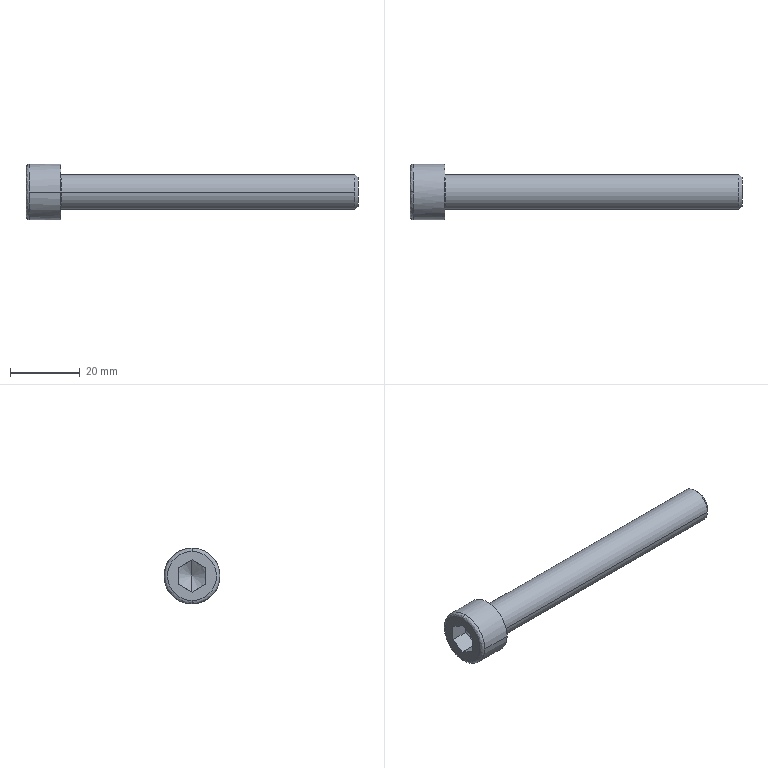Part | STEP file | AS 1420 - Metric M10 x 45_2 | 1 solid | 21 faces | box 95 x 16 x 16 mm | volume 8328 mm3 | plane 9 | spline 4 | cylinder 4 | cone 4 | commonest cylinder face diameters 10 x2 16 x2